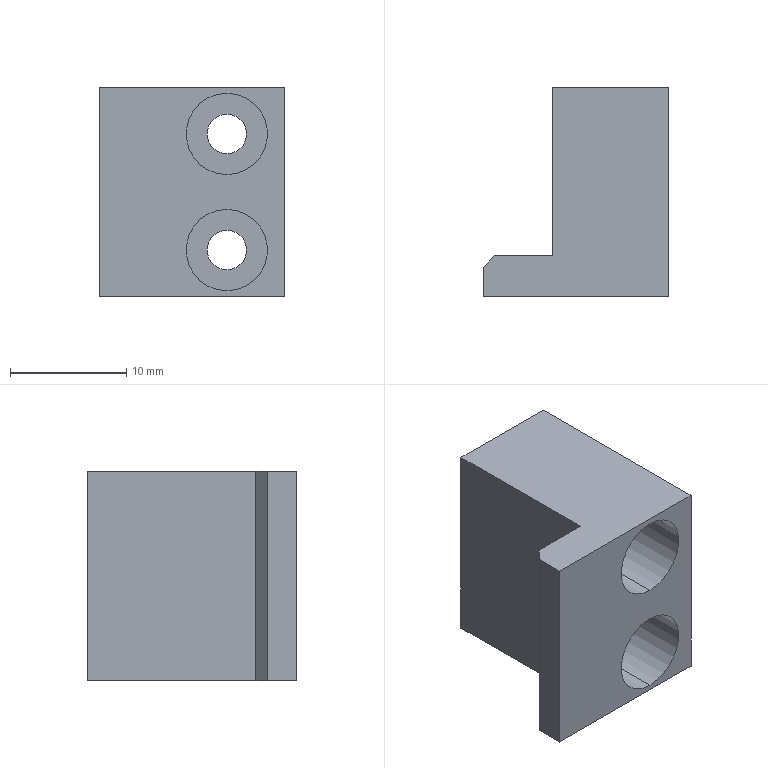Part | NX | features BREP 1 | 1 solid | 19 faces | box 16 x 18 x 18 mm | volume 2576 mm3 | plane 11 | cylinder 8 | commonest cylinder face diameters 3.4 x4 7 x4
STEP:
#1=CARTESIAN_POINT('',(-5.,0.,9.));
#2=VERTEX_POINT('',#1);
#3=CARTESIAN_POINT('',(-6.,-1.,9.));
#4=VERTEX_POINT('',#3);
#5=CARTESIAN_POINT('',(-6.,-1.,9.));
#6=DIRECTION('',(-0.7071,-0.7071,0.));
#7=VECTOR('',#6,1000.);
#8=LINE('',#5,#7);
#9=EDGE_CURVE('',#2,#4,#8,.T.);
#10=ORIENTED_EDGE('',*,*,#9,.F.);
#11=CARTESIAN_POINT('',(-5.,0.,-9.));
#12=VERTEX_POINT('',#11);
#13=CARTESIAN_POINT('',(-5.,0.,9.));
#14=DIRECTION('',(0.,0.,1.));
#15=VECTOR('',#14,1000.);
#16=LINE('',#13,#15);
#17=EDGE_CURVE('',#12,#2,#16,.T.);
#18=ORIENTED_EDGE('',*,*,#17,.F.);
#19=CARTESIAN_POINT('',(-6.,-1.,-9.));
#20=VERTEX_POINT('',#19);
#21=CARTESIAN_POINT('',(-2.5,2.5,-9.));
#22=DIRECTION('',(0.7071,0.7071,0.));
#23=VECTOR('',#22,1000.);
#24=LINE('',#21,#23);
#25=EDGE_CURVE('',#20,#12,#24,.T.);
#26=ORIENTED_EDGE('',*,*,#25,.F.);
#27=CARTESIAN_POINT('',(-6.,-1.,9.));
#28=DIRECTION('',(0.,0.,-1.));
#29=VECTOR('',#28,1000.);
#30=LINE('',#27,#29);
#31=EDGE_CURVE('',#4,#20,#30,.T.);
#32=ORIENTED_EDGE('',*,*,#31,.F.);
#33=EDGE_LOOP('',(#10,#18,#26,#32));
#34=FACE_BOUND('',#33,.T.);
#35=CARTESIAN_POINT('',(-6.,-1.,9.));
#36=DIRECTION('',(0.7071,-0.7071,0.));
#37=DIRECTION('',(0.,0.,-1.));
#38=AXIS2_PLACEMENT_3D('',#35,#36,#37);
#39=PLANE('',#38);
#40=ADVANCED_FACE('',(#34),#39,.F.);
#41=CARTESIAN_POINT('',(5.,8.5,8.5));
#42=VERTEX_POINT('',#41);
#43=CARTESIAN_POINT('',(5.,-3.5,8.5));
#44=VERTEX_POINT('',#43);
#45=CARTESIAN_POINT('',(5.,-3.5,8.5));
#46=DIRECTION('',(0.,-1.,0.));
#47=VECTOR('',#46,1000.);
#48=LINE('',#45,#47);
#49=EDGE_CURVE('',#42,#44,#48,.T.);
#50=ORIENTED_EDGE('',*,*,#49,.F.);
#51=CARTESIAN_POINT('',(5.,8.5,1.5));
#52=VERTEX_POINT('',#51);
#53=CARTESIAN_POINT('',(5.,8.5,5.));
#54=DIRECTION('',(0.,-1.,0.));
#55=DIRECTION('',(0.,0.,-1.));
#56=AXIS2_PLACEMENT_3D('',#53,#54,#55);
#57=CIRCLE('',#56,3.5);
#58=EDGE_CURVE('',#52,#42,#57,.T.);
#59=ORIENTED_EDGE('',*,*,#58,.F.);
#60=CARTESIAN_POINT('',(5.,-3.5,1.5));
#61=VERTEX_POINT('',#60);
#62=CARTESIAN_POINT('',(5.,-3.5,1.5));
#63=DIRECTION('',(0.,-1.,0.));
#64=VECTOR('',#63,1000.);
#65=LINE('',#62,#64);
#66=EDGE_CURVE('',#52,#61,#65,.T.);
#67=ORIENTED_EDGE('',*,*,#66,.T.);
#68=CARTESIAN_POINT('',(5.,-3.5,5.));
#69=DIRECTION('',(0.,-1.,0.));
#70=DIRECTION('',(0.,0.,-1.));
#71=AXIS2_PLACEMENT_3D('',#68,#69,#70);
#72=CIRCLE('',#71,3.5);
#73=EDGE_CURVE('',#61,#44,#72,.T.);
#74=ORIENTED_EDGE('',*,*,#73,.T.);
#75=EDGE_LOOP('',(#50,#59,#67,#74));
#76=FACE_BOUND('',#75,.T.);
#77=CARTESIAN_POINT('',(5.,-3.5,5.));
#78=DIRECTION('',(0.,-1.,0.));
#79=DIRECTION('',(0.,0.,-1.));
#80=AXIS2_PLACEMENT_3D('',#77,#78,#79);
#81=CYLINDRICAL_SURFACE('',#80,3.5);
#82=ADVANCED_FACE('',(#76),#81,.F.);
#83=ORIENTED_EDGE('',*,*,#58,.T.);
#84=CARTESIAN_POINT('',(5.,8.5,5.));
#85=DIRECTION('',(0.,-1.,0.));
#86=DIRECTION('',(0.,0.,-1.));
#87=AXIS2_PLACEMENT_3D('',#84,#85,#86);
#88=CIRCLE('',#87,3.5);
#89=EDGE_CURVE('',#42,#52,#88,.T.);
#90=ORIENTED_EDGE('',*,*,#89,.T.);
#91=EDGE_LOOP('',(#83,#90));
#92=FACE_BOUND('',#91,.T.);
#93=CARTESIAN_POINT('',(5.,8.5,3.3));
#94=VERTEX_POINT('',#93);
#95=CARTESIAN_POINT('',(5.,8.5,6.7));
#96=VERTEX_POINT('',#95);
#97=CARTESIAN_POINT('',(5.,8.5,5.));
#98=DIRECTION('',(0.,-1.,0.));
#99=DIRECTION('',(0.,0.,-1.));
#100=AXIS2_PLACEMENT_3D('',#97,#98,#99);
#101=CIRCLE('',#100,1.7);
#102=EDGE_CURVE('',#94,#96,#101,.T.);
#103=ORIENTED_EDGE('',*,*,#102,.F.);
#104=CARTESIAN_POINT('',(5.,8.5,5.));
#105=DIRECTION('',(0.,-1.,0.));
#106=DIRECTION('',(0.,0.,-1.));
#107=AXIS2_PLACEMENT_3D('',#104,#105,#106);
#108=CIRCLE('',#107,1.7);
#109=EDGE_CURVE('',#96,#94,#108,.T.);
#110=ORIENTED_EDGE('',*,*,#109,.F.);
#111=EDGE_LOOP('',(#103,#110));
#112=FACE_BOUND('',#111,.T.);
#113=CARTESIAN_POINT('',(6.7,8.5,5.));
#114=DIRECTION('',(0.,1.,0.));
#115=DIRECTION('',(0.,0.,1.));
#116=AXIS2_PLACEMENT_3D('',#113,#114,#115);
#117=PLANE('',#116);
#118=ADVANCED_FACE('',(#92,#112),#117,.F.);
#119=CARTESIAN_POINT('',(5.,14.5,6.7));
#120=VERTEX_POINT('',#119);
#121=CARTESIAN_POINT('',(5.,-3.5,6.7));
#122=DIRECTION('',(0.,-1.,0.));
#123=VECTOR('',#122,1000.);
#124=LINE('',#121,#123);
#125=EDGE_CURVE('',#120,#96,#124,.T.);
#126=ORIENTED_EDGE('',*,*,#125,.F.);
#127=CARTESIAN_POINT('',(5.,14.5,3.3));
#128=VERTEX_POINT('',#127);
#129=CARTESIAN_POINT('',(5.,14.5,5.));
#130=DIRECTION('',(0.,-1.,0.));
#131=DIRECTION('',(0.,0.,-1.));
#132=AXIS2_PLACEMENT_3D('',#129,#130,#131);
#133=CIRCLE('',#132,1.7);
#134=EDGE_CURVE('',#128,#120,#133,.T.);
#135=ORIENTED_EDGE('',*,*,#134,.F.);
#136=CARTESIAN_POINT('',(5.,-3.5,3.3));
#137=DIRECTION('',(0.,-1.,0.));
#138=VECTOR('',#137,1000.);
#139=LINE('',#136,#138);
#140=EDGE_CURVE('',#128,#94,#139,.T.);
#141=ORIENTED_EDGE('',*,*,#140,.T.);
#142=ORIENTED_EDGE('',*,*,#102,.T.);
#143=EDGE_LOOP('',(#126,#135,#141,#142));
#144=FACE_BOUND('',#143,.T.);
#145=CARTESIAN_POINT('',(5.,-3.5,5.));
#146=DIRECTION('',(0.,-1.,0.));
#147=DIRECTION('',(0.,0.,-1.));
#148=AXIS2_PLACEMENT_3D('',#145,#146,#147);
#149=CYLINDRICAL_SURFACE('',#148,1.7);
#150=ADVANCED_FACE('',(#144),#149,.F.);
#151=CARTESIAN_POINT('',(5.,8.5,-1.5));
#152=VERTEX_POINT('',#151);
#153=CARTESIAN_POINT('',(5.,-3.5,-1.5));
#154=VERTEX_POINT('',#153);
#155=CARTESIAN_POINT('',(5.,-3.5,-1.5));
#156=DIRECTION('',(0.,-1.,0.));
#157=VECTOR('',#156,1000.);
#158=LINE('',#155,#157);
#159=EDGE_CURVE('',#152,#154,#158,.T.);
#160=ORIENTED_EDGE('',*,*,#159,.F.);
#161=CARTESIAN_POINT('',(5.,8.5,-8.5));
#162=VERTEX_POINT('',#161);
#163=CARTESIAN_POINT('',(5.,8.5,-5.));
#164=DIRECTION('',(0.,-1.,0.));
#165=DIRECTION('',(0.,0.,-1.));
#166=AXIS2_PLACEMENT_3D('',#163,#164,#165);
#167=CIRCLE('',#166,3.5);
#168=EDGE_CURVE('',#162,#152,#167,.T.);
#169=ORIENTED_EDGE('',*,*,#168,.F.);
#170=CARTESIAN_POINT('',(5.,-3.5,-8.5));
#171=VERTEX_POINT('',#170);
#172=CARTESIAN_POINT('',(5.,-3.5,-8.5));
#173=DIRECTION('',(0.,-1.,0.));
#174=VECTOR('',#173,1000.);
#175=LINE('',#172,#174);
#176=EDGE_CURVE('',#162,#171,#175,.T.);
#177=ORIENTED_EDGE('',*,*,#176,.T.);
#178=CARTESIAN_POINT('',(5.,-3.5,-5.));
#179=DIRECTION('',(0.,-1.,0.));
#180=DIRECTION('',(0.,0.,-1.));
#181=AXIS2_PLACEMENT_3D('',#178,#179,#180);
#182=CIRCLE('',#181,3.5);
#183=EDGE_CURVE('',#171,#154,#182,.T.);
#184=ORIENTED_EDGE('',*,*,#183,.T.);
#185=EDGE_LOOP('',(#160,#169,#177,#184));
#186=FACE_BOUND('',#185,.T.);
#187=CARTESIAN_POINT('',(5.,-3.5,-5.));
#188=DIRECTION('',(0.,-1.,0.));
#189=DIRECTION('',(0.,0.,-1.));
#190=AXIS2_PLACEMENT_3D('',#187,#188,#189);
#191=CYLINDRICAL_SURFACE('',#190,3.5);
#192=ADVANCED_FACE('',(#186),#191,.F.);
#193=ORIENTED_EDGE('',*,*,#168,.T.);
#194=CARTESIAN_POINT('',(5.,8.5,-5.));
#195=DIRECTION('',(0.,-1.,0.));
#196=DIRECTION('',(0.,0.,-1.));
#197=AXIS2_PLACEMENT_3D('',#194,#195,#196);
#198=CIRCLE('',#197,3.5);
#199=EDGE_CURVE('',#152,#162,#198,.T.);
#200=ORIENTED_EDGE('',*,*,#199,.T.);
#201=EDGE_LOOP('',(#193,#200));
#202=FACE_BOUND('',#201,.T.);
#203=CARTESIAN_POINT('',(5.,8.5,-6.7));
#204=VERTEX_POINT('',#203);
#205=CARTESIAN_POINT('',(5.,8.5,-3.3));
#206=VERTEX_POINT('',#205);
#207=CARTESIAN_POINT('',(5.,8.5,-5.));
#208=DIRECTION('',(0.,-1.,0.));
#209=DIRECTION('',(0.,0.,-1.));
#210=AXIS2_PLACEMENT_3D('',#207,#208,#209);
#211=CIRCLE('',#210,1.7);
#212=EDGE_CURVE('',#204,#206,#211,.T.);
#213=ORIENTED_EDGE('',*,*,#212,.F.);
#214=CARTESIAN_POINT('',(5.,8.5,-5.));
#215=DIRECTION('',(0.,-1.,0.));
#216=DIRECTION('',(0.,0.,-1.));
#217=AXIS2_PLACEMENT_3D('',#214,#215,#216);
#218=CIRCLE('',#217,1.7);
#219=EDGE_CURVE('',#206,#204,#218,.T.);
#220=ORIENTED_EDGE('',*,*,#219,.F.);
#221=EDGE_LOOP('',(#213,#220));
#222=FACE_BOUND('',#221,.T.);
#223=CARTESIAN_POINT('',(6.7,8.5,-5.));
#224=DIRECTION('',(0.,1.,0.));
#225=DIRECTION('',(0.,0.,1.));
#226=AXIS2_PLACEMENT_3D('',#223,#224,#225);
#227=PLANE('',#226);
#228=ADVANCED_FACE('',(#202,#222),#227,.F.);
#229=CARTESIAN_POINT('',(5.,14.5,-3.3));
#230=VERTEX_POINT('',#229);
#231=CARTESIAN_POINT('',(5.,-3.5,-3.3));
#232=DIRECTION('',(0.,-1.,0.));
#233=VECTOR('',#232,1000.);
#234=LINE('',#231,#233);
#235=EDGE_CURVE('',#230,#206,#234,.T.);
#236=ORIENTED_EDGE('',*,*,#235,.F.);
#237=CARTESIAN_POINT('',(5.,14.5,-6.7));
#238=VERTEX_POINT('',#237);
#239=CARTESIAN_POINT('',(5.,14.5,-5.));
#240=DIRECTION('',(0.,-1.,0.));
#241=DIRECTION('',(0.,0.,-1.));
#242=AXIS2_PLACEMENT_3D('',#239,#240,#241);
#243=CIRCLE('',#242,1.7);
#244=EDGE_CURVE('',#238,#230,#243,.T.);
#245=ORIENTED_EDGE('',*,*,#244,.F.);
#246=CARTESIAN_POINT('',(5.,-3.5,-6.7));
#247=DIRECTION('',(0.,-1.,0.));
#248=VECTOR('',#247,1000.);
#249=LINE('',#246,#248);
#250=EDGE_CURVE('',#238,#204,#249,.T.);
#251=ORIENTED_EDGE('',*,*,#250,.T.);
#252=ORIENTED_EDGE('',*,*,#212,.T.);
#253=EDGE_LOOP('',(#236,#245,#251,#252));
#254=FACE_BOUND('',#253,.T.);
#255=CARTESIAN_POINT('',(5.,-3.5,-5.));
#256=DIRECTION('',(0.,-1.,0.));
#257=DIRECTION('',(0.,0.,-1.));
#258=AXIS2_PLACEMENT_3D('',#255,#256,#257);
#259=CYLINDRICAL_SURFACE('',#258,1.7);
#260=ADVANCED_FACE('',(#254),#259,.F.);
#261=CARTESIAN_POINT('',(-6.,-3.5,-9.));
#262=VERTEX_POINT('',#261);
#263=CARTESIAN_POINT('',(-6.,0.,-9.));
#264=DIRECTION('',(0.,-1.,0.));
#265=VECTOR('',#264,1000.);
#266=LINE('',#263,#265);
#267=EDGE_CURVE('',#20,#262,#266,.T.);
#268=ORIENTED_EDGE('',*,*,#267,.F.);
#269=ORIENTED_EDGE('',*,*,#25,.T.);
#270=CARTESIAN_POINT('',(0.,0.,-9.));
#271=VERTEX_POINT('',#270);
#272=CARTESIAN_POINT('',(0.,0.,-9.));
#273=DIRECTION('',(-1.,0.,0.));
#274=VECTOR('',#273,1000.);
#275=LINE('',#272,#274);
#276=EDGE_CURVE('',#271,#12,#275,.T.);
#277=ORIENTED_EDGE('',*,*,#276,.F.);
#278=CARTESIAN_POINT('',(0.,14.5,-9.));
#279=VERTEX_POINT('',#278);
#280=CARTESIAN_POINT('',(0.,14.5,-9.));
#281=DIRECTION('',(0.,-1.,0.));
#282=VECTOR('',#281,1000.);
#283=LINE('',#280,#282);
#284=EDGE_CURVE('',#279,#271,#283,.T.);
#285=ORIENTED_EDGE('',*,*,#284,.F.);
#286=CARTESIAN_POINT('',(10.,14.5,-9.));
#287=VERTEX_POINT('',#286);
#288=CARTESIAN_POINT('',(10.,14.5,-9.));
#289=DIRECTION('',(-1.,0.,0.));
#290=VECTOR('',#289,1000.);
#291=LINE('',#288,#290);
#292=EDGE_CURVE('',#287,#279,#291,.T.);
#293=ORIENTED_EDGE('',*,*,#292,.F.);
#294=CARTESIAN_POINT('',(10.,-3.5,-9.));
#295=VERTEX_POINT('',#294);
#296=CARTESIAN_POINT('',(10.,-3.5,-9.));
#297=DIRECTION('',(0.,1.,0.));
#298=VECTOR('',#297,1000.);
#299=LINE('',#296,#298);
#300=EDGE_CURVE('',#295,#287,#299,.T.);
#301=ORIENTED_EDGE('',*,*,#300,.F.);
#302=CARTESIAN_POINT('',(-6.,-3.5,-9.));
#303=DIRECTION('',(1.,0.,0.));
#304=VECTOR('',#303,1000.);
#305=LINE('',#302,#304);
#306=EDGE_CURVE('',#262,#295,#305,.T.);
#307=ORIENTED_EDGE('',*,*,#306,.F.);
#308=EDGE_LOOP('',(#268,#269,#277,#285,#293,#301,#307));
#309=FACE_BOUND('',#308,.T.);
#310=CARTESIAN_POINT('',(0.,0.,-9.));
#311=DIRECTION('',(0.,0.,-1.));
#312=DIRECTION('',(-1.,0.,0.));
#313=AXIS2_PLACEMENT_3D('',#310,#311,#312);
#314=PLANE('',#313);
#315=ADVANCED_FACE('',(#309),#314,.T.);
#316=CARTESIAN_POINT('',(0.,0.,9.));
#317=VERTEX_POINT('',#316);
#318=CARTESIAN_POINT('',(0.,0.,9.));
#319=DIRECTION('',(-1.,0.,0.));
#320=VECTOR('',#319,1000.);
#321=LINE('',#318,#320);
#322=EDGE_CURVE('',#317,#2,#321,.T.);
#323=ORIENTED_EDGE('',*,*,#322,.T.);
#324=ORIENTED_EDGE('',*,*,#9,.T.);
#325=CARTESIAN_POINT('',(-6.,-3.5,9.));
#326=VERTEX_POINT('',#325);
#327=CARTESIAN_POINT('',(-6.,0.,9.));
#328=DIRECTION('',(0.,-1.,0.));
#329=VECTOR('',#328,1000.);
#330=LINE('',#327,#329);
#331=EDGE_CURVE('',#4,#326,#330,.T.);
#332=ORIENTED_EDGE('',*,*,#331,.T.);
#333=CARTESIAN_POINT('',(10.,-3.5,9.));
#334=VERTEX_POINT('',#333);
#335=CARTESIAN_POINT('',(-6.,-3.5,9.));
#336=DIRECTION('',(1.,0.,0.));
#337=VECTOR('',#336,1000.);
#338=LINE('',#335,#337);
#339=EDGE_CURVE('',#326,#334,#338,.T.);
#340=ORIENTED_EDGE('',*,*,#339,.T.);
#341=CARTESIAN_POINT('',(10.,14.5,9.));
#342=VERTEX_POINT('',#341);
#343=CARTESIAN_POINT('',(10.,-3.5,9.));
#344=DIRECTION('',(0.,1.,0.));
#345=VECTOR('',#344,1000.);
#346=LINE('',#343,#345);
#347=EDGE_CURVE('',#334,#342,#346,.T.);
#348=ORIENTED_EDGE('',*,*,#347,.T.);
#349=CARTESIAN_POINT('',(0.,14.5,9.));
#350=VERTEX_POINT('',#349);
#351=CARTESIAN_POINT('',(10.,14.5,9.));
#352=DIRECTION('',(-1.,0.,0.));
#353=VECTOR('',#352,1000.);
#354=LINE('',#351,#353);
#355=EDGE_CURVE('',#342,#350,#354,.T.);
#356=ORIENTED_EDGE('',*,*,#355,.T.);
#357=CARTESIAN_POINT('',(0.,14.5,9.));
#358=DIRECTION('',(0.,-1.,0.));
#359=VECTOR('',#358,1000.);
#360=LINE('',#357,#359);
#361=EDGE_CURVE('',#350,#317,#360,.T.);
#362=ORIENTED_EDGE('',*,*,#361,.T.);
#363=EDGE_LOOP('',(#323,#324,#332,#340,#348,#356,#362));
#364=FACE_BOUND('',#363,.T.);
#365=CARTESIAN_POINT('',(0.,0.,9.));
#366=DIRECTION('',(0.,0.,-1.));
#367=DIRECTION('',(-1.,0.,0.));
#368=AXIS2_PLACEMENT_3D('',#365,#366,#367);
#369=PLANE('',#368);
#370=ADVANCED_FACE('',(#364),#369,.F.);
#371=ORIENTED_EDGE('',*,*,#292,.T.);
#372=CARTESIAN_POINT('',(0.,14.5,9.));
#373=DIRECTION('',(0.,0.,-1.));
#374=VECTOR('',#373,1000.);
#375=LINE('',#372,#374);
#376=EDGE_CURVE('',#350,#279,#375,.T.);
#377=ORIENTED_EDGE('',*,*,#376,.F.);
#378=ORIENTED_EDGE('',*,*,#355,.F.);
#379=CARTESIAN_POINT('',(10.,14.5,9.));
#380=DIRECTION('',(0.,0.,-1.));
#381=VECTOR('',#380,1000.);
#382=LINE('',#379,#381);
#383=EDGE_CURVE('',#342,#287,#382,.T.);
#384=ORIENTED_EDGE('',*,*,#383,.T.);
#385=EDGE_LOOP('',(#371,#377,#378,#384));
#386=FACE_BOUND('',#385,.T.);
#387=ORIENTED_EDGE('',*,*,#244,.T.);
#388=CARTESIAN_POINT('',(5.,14.5,-5.));
#389=DIRECTION('',(0.,-1.,0.));
#390=DIRECTION('',(0.,0.,-1.));
#391=AXIS2_PLACEMENT_3D('',#388,#389,#390);
#392=CIRCLE('',#391,1.7);
#393=EDGE_CURVE('',#230,#238,#392,.T.);
#394=ORIENTED_EDGE('',*,*,#393,.T.);
#395=EDGE_LOOP('',(#387,#394));
#396=FACE_BOUND('',#395,.T.);
#397=ORIENTED_EDGE('',*,*,#134,.T.);
#398=CARTESIAN_POINT('',(5.,14.5,5.));
#399=DIRECTION('',(0.,-1.,0.));
#400=DIRECTION('',(0.,0.,-1.));
#401=AXIS2_PLACEMENT_3D('',#398,#399,#400);
#402=CIRCLE('',#401,1.7);
#403=EDGE_CURVE('',#120,#128,#402,.T.);
#404=ORIENTED_EDGE('',*,*,#403,.T.);
#405=EDGE_LOOP('',(#397,#404));
#406=FACE_BOUND('',#405,.T.);
#407=CARTESIAN_POINT('',(10.,14.5,9.));
#408=DIRECTION('',(0.,-1.,0.));
#409=DIRECTION('',(0.,0.,-1.));
#410=AXIS2_PLACEMENT_3D('',#407,#408,#409);
#411=PLANE('',#410);
#412=ADVANCED_FACE('',(#386,#396,#406),#411,.F.);
#413=ORIENTED_EDGE('',*,*,#300,.T.);
#414=ORIENTED_EDGE('',*,*,#383,.F.);
#415=ORIENTED_EDGE('',*,*,#347,.F.);
#416=CARTESIAN_POINT('',(10.,-3.5,9.));
#417=DIRECTION('',(0.,0.,-1.));
#418=VECTOR('',#417,1000.);
#419=LINE('',#416,#418);
#420=EDGE_CURVE('',#334,#295,#419,.T.);
#421=ORIENTED_EDGE('',*,*,#420,.T.);
#422=EDGE_LOOP('',(#413,#414,#415,#421));
#423=FACE_BOUND('',#422,.T.);
#424=CARTESIAN_POINT('',(10.,-3.5,9.));
#425=DIRECTION('',(-1.,0.,0.));
#426=DIRECTION('',(0.,-1.,0.));
#427=AXIS2_PLACEMENT_3D('',#424,#425,#426);
#428=PLANE('',#427);
#429=ADVANCED_FACE('',(#423),#428,.F.);
#430=ORIENTED_EDGE('',*,*,#306,.T.);
#431=ORIENTED_EDGE('',*,*,#420,.F.);
#432=ORIENTED_EDGE('',*,*,#339,.F.);
#433=CARTESIAN_POINT('',(-6.,-3.5,9.));
#434=DIRECTION('',(0.,0.,-1.));
#435=VECTOR('',#434,1000.);
#436=LINE('',#433,#435);
#437=EDGE_CURVE('',#326,#262,#436,.T.);
#438=ORIENTED_EDGE('',*,*,#437,.T.);
#439=EDGE_LOOP('',(#430,#431,#432,#438));
#440=FACE_BOUND('',#439,.T.);
#441=ORIENTED_EDGE('',*,*,#183,.F.);
#442=CARTESIAN_POINT('',(5.,-3.5,-5.));
#443=DIRECTION('',(0.,-1.,0.));
#444=DIRECTION('',(0.,0.,-1.));
#445=AXIS2_PLACEMENT_3D('',#442,#443,#444);
#446=CIRCLE('',#445,3.5);
#447=EDGE_CURVE('',#154,#171,#446,.T.);
#448=ORIENTED_EDGE('',*,*,#447,.F.);
#449=EDGE_LOOP('',(#441,#448));
#450=FACE_BOUND('',#449,.T.);
#451=ORIENTED_EDGE('',*,*,#73,.F.);
#452=CARTESIAN_POINT('',(5.,-3.5,5.));
#453=DIRECTION('',(0.,-1.,0.));
#454=DIRECTION('',(0.,0.,-1.));
#455=AXIS2_PLACEMENT_3D('',#452,#453,#454);
#456=CIRCLE('',#455,3.5);
#457=EDGE_CURVE('',#44,#61,#456,.T.);
#458=ORIENTED_EDGE('',*,*,#457,.F.);
#459=EDGE_LOOP('',(#451,#458));
#460=FACE_BOUND('',#459,.T.);
#461=CARTESIAN_POINT('',(-6.,-3.5,9.));
#462=DIRECTION('',(0.,1.,0.));
#463=DIRECTION('',(-1.,0.,0.));
#464=AXIS2_PLACEMENT_3D('',#461,#462,#463);
#465=PLANE('',#464);
#466=ADVANCED_FACE('',(#440,#450,#460),#465,.F.);
#467=ORIENTED_EDGE('',*,*,#331,.F.);
#468=ORIENTED_EDGE('',*,*,#31,.T.);
#469=ORIENTED_EDGE('',*,*,#267,.T.);
#470=ORIENTED_EDGE('',*,*,#437,.F.);
#471=EDGE_LOOP('',(#467,#468,#469,#470));
#472=FACE_BOUND('',#471,.T.);
#473=CARTESIAN_POINT('',(-6.,0.,9.));
#474=DIRECTION('',(1.,0.,0.));
#475=DIRECTION('',(0.,0.,-1.));
#476=AXIS2_PLACEMENT_3D('',#473,#474,#475);
#477=PLANE('',#476);
#478=ADVANCED_FACE('',(#472),#477,.F.);
#479=ORIENTED_EDGE('',*,*,#276,.T.);
#480=ORIENTED_EDGE('',*,*,#17,.T.);
#481=ORIENTED_EDGE('',*,*,#322,.F.);
#482=CARTESIAN_POINT('',(0.,0.,9.));
#483=DIRECTION('',(0.,0.,-1.));
#484=VECTOR('',#483,1000.);
#485=LINE('',#482,#484);
#486=EDGE_CURVE('',#317,#271,#485,.T.);
#487=ORIENTED_EDGE('',*,*,#486,.T.);
#488=EDGE_LOOP('',(#479,#480,#481,#487));
#489=FACE_BOUND('',#488,.T.);
#490=CARTESIAN_POINT('',(0.,0.,9.));
#491=DIRECTION('',(0.,-1.,0.));
#492=DIRECTION('',(1.,0.,0.));
#493=AXIS2_PLACEMENT_3D('',#490,#491,#492);
#494=PLANE('',#493);
#495=ADVANCED_FACE('',(#489),#494,.F.);
#496=ORIENTED_EDGE('',*,*,#284,.T.);
#497=ORIENTED_EDGE('',*,*,#486,.F.);
#498=ORIENTED_EDGE('',*,*,#361,.F.);
#499=ORIENTED_EDGE('',*,*,#376,.T.);
#500=EDGE_LOOP('',(#496,#497,#498,#499));
#501=FACE_BOUND('',#500,.T.);
#502=CARTESIAN_POINT('',(0.,14.5,9.));
#503=DIRECTION('',(1.,0.,0.));
#504=DIRECTION('',(0.,0.,-1.));
#505=AXIS2_PLACEMENT_3D('',#502,#503,#504);
#506=PLANE('',#505);
#507=ADVANCED_FACE('',(#501),#506,.F.);
#508=ORIENTED_EDGE('',*,*,#393,.F.);
#509=ORIENTED_EDGE('',*,*,#235,.T.);
#510=ORIENTED_EDGE('',*,*,#219,.T.);
#511=ORIENTED_EDGE('',*,*,#250,.F.);
#512=EDGE_LOOP('',(#508,#509,#510,#511));
#513=FACE_BOUND('',#512,.T.);
#514=CARTESIAN_POINT('',(5.,-3.5,-5.));
#515=DIRECTION('',(0.,-1.,0.));
#516=DIRECTION('',(0.,0.,-1.));
#517=AXIS2_PLACEMENT_3D('',#514,#515,#516);
#518=CYLINDRICAL_SURFACE('',#517,1.7);
#519=ADVANCED_FACE('',(#513),#518,.F.);
#520=ORIENTED_EDGE('',*,*,#199,.F.);
#521=ORIENTED_EDGE('',*,*,#159,.T.);
#522=ORIENTED_EDGE('',*,*,#447,.T.);
#523=ORIENTED_EDGE('',*,*,#176,.F.);
#524=EDGE_LOOP('',(#520,#521,#522,#523));
#525=FACE_BOUND('',#524,.T.);
#526=CARTESIAN_POINT('',(5.,-3.5,-5.));
#527=DIRECTION('',(0.,-1.,0.));
#528=DIRECTION('',(0.,0.,-1.));
#529=AXIS2_PLACEMENT_3D('',#526,#527,#528);
#530=CYLINDRICAL_SURFACE('',#529,3.5);
#531=ADVANCED_FACE('',(#525),#530,.F.);
#532=ORIENTED_EDGE('',*,*,#403,.F.);
#533=ORIENTED_EDGE('',*,*,#125,.T.);
#534=ORIENTED_EDGE('',*,*,#109,.T.);
#535=ORIENTED_EDGE('',*,*,#140,.F.);
#536=EDGE_LOOP('',(#532,#533,#534,#535));
#537=FACE_BOUND('',#536,.T.);
#538=CARTESIAN_POINT('',(5.,-3.5,5.));
#539=DIRECTION('',(0.,-1.,0.));
#540=DIRECTION('',(0.,0.,-1.));
#541=AXIS2_PLACEMENT_3D('',#538,#539,#540);
#542=CYLINDRICAL_SURFACE('',#541,1.7);
#543=ADVANCED_FACE('',(#537),#542,.F.);
#544=ORIENTED_EDGE('',*,*,#89,.F.);
#545=ORIENTED_EDGE('',*,*,#49,.T.);
#546=ORIENTED_EDGE('',*,*,#457,.T.);
#547=ORIENTED_EDGE('',*,*,#66,.F.);
#548=EDGE_LOOP('',(#544,#545,#546,#547));
#549=FACE_BOUND('',#548,.T.);
#550=CARTESIAN_POINT('',(5.,-3.5,5.));
#551=DIRECTION('',(0.,-1.,0.));
#552=DIRECTION('',(0.,0.,-1.));
#553=AXIS2_PLACEMENT_3D('',#550,#551,#552);
#554=CYLINDRICAL_SURFACE('',#553,3.5);
#555=ADVANCED_FACE('',(#549),#554,.F.);
#556=CLOSED_SHELL('',(#40,#82,#118,#150,#192,#228,#260,#315,#370,#412,#429,#466,#478,#495,#507,#519,#531,#543,#555));
#557=MANIFOLD_SOLID_BREP('',#556);
#558=(LENGTH_UNIT()NAMED_UNIT(*)SI_UNIT(.MILLI.,.METRE.));
#559=UNCERTAINTY_MEASURE_WITH_UNIT(LENGTH_MEASURE(0.00001),#558,'','');
#560=(NAMED_UNIT(*)PLANE_ANGLE_UNIT()SI_UNIT($,.RADIAN.));
#561=(NAMED_UNIT(*)SI_UNIT($,.STERADIAN.)SOLID_ANGLE_UNIT());
#562=(GEOMETRIC_REPRESENTATION_CONTEXT(3)GLOBAL_UNCERTAINTY_ASSIGNED_CONTEXT((#559))GLOBAL_UNIT_ASSIGNED_CONTEXT((#558,#560,#561))REPRESENTATION_CONTEXT('',''));
#563=ADVANCED_BREP_SHAPE_REPRESENTATION('',(#557),#562);